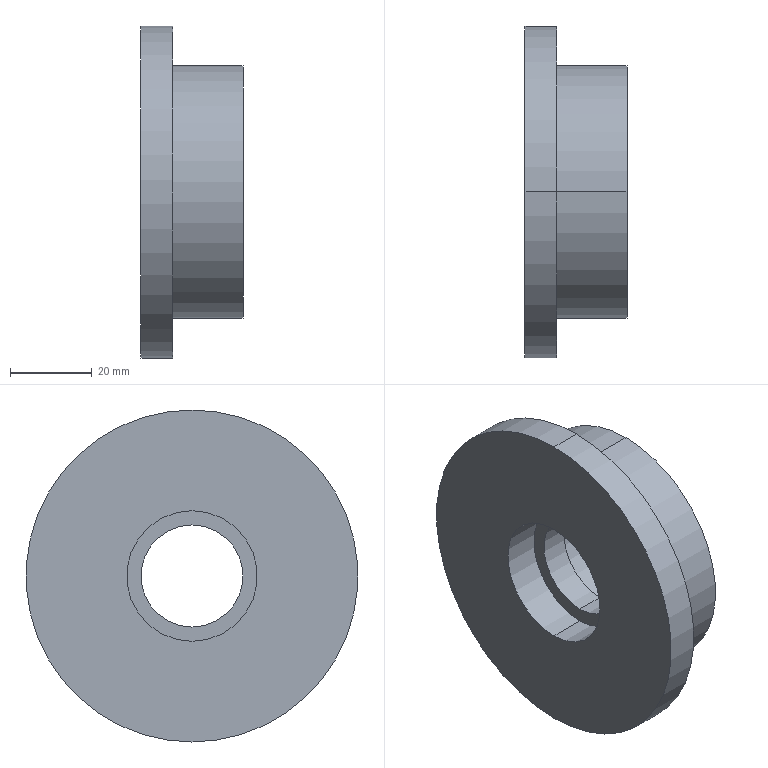Part | STEP file | PN_0073 (sprocket z=16,p=15.875) | 1 solid | 15 faces | box 25 x 81.37 x 81.37 mm | volume 74577 mm3 | cylinder 10 | plane 5 | commonest cylinder face diameters 32 x4 25 x2 62 x2 81.37 x2
STEP:
#1=CARTESIAN_POINT('',(0.,0.,0.));
#2=DIRECTION('',(0.,0.,1.));
#3=DIRECTION('',(1.,0.,0.));
#4=AXIS2_PLACEMENT_3D('',#1,#2,#3);
#5=CARTESIAN_POINT('',(9.,0.,16.));
#6=VERTEX_POINT('',#5);
#7=CARTESIAN_POINT('',(0.,0.,16.));
#8=VERTEX_POINT('',#7);
#9=CARTESIAN_POINT('',(9.,0.,16.));
#10=DIRECTION('',(-1.,0.,0.));
#11=VECTOR('',#10,1.);
#12=LINE('',#9,#11);
#13=CARTESIAN_POINT('',(9.,0.,0.));
#14=DIRECTION('',(-1.,0.,0.));
#15=DIRECTION('',(0.,0.,1.));
#16=AXIS2_PLACEMENT_3D('',#13,#14,#15);
#17=CYLINDRICAL_SURFACE('',#16,16.);
#18=CARTESIAN_POINT('',(6.283,0.));
#19=DIRECTION('',(0.,1.));
#20=VECTOR('',#19,1.);
#21=LINE('',#18,#20);
#22=(GEOMETRIC_REPRESENTATION_CONTEXT(2)PARAMETRIC_REPRESENTATION_CONTEXT()REPRESENTATION_CONTEXT('',''));
#23=DEFINITIONAL_REPRESENTATION('',(#21),#22);
#24=PCURVE('',#17,#23);
#25=CARTESIAN_POINT('',(9.,0.,0.));
#26=DIRECTION('',(-1.,0.,0.));
#27=DIRECTION('',(0.,0.,1.));
#28=AXIS2_PLACEMENT_3D('',#25,#26,#27);
#29=CYLINDRICAL_SURFACE('',#28,16.);
#30=CARTESIAN_POINT('',(0.,0.));
#31=DIRECTION('',(0.,1.));
#32=VECTOR('',#31,1.);
#33=LINE('',#30,#32);
#34=(GEOMETRIC_REPRESENTATION_CONTEXT(2)PARAMETRIC_REPRESENTATION_CONTEXT()REPRESENTATION_CONTEXT('',''));
#35=DEFINITIONAL_REPRESENTATION('',(#33),#34);
#36=PCURVE('',#29,#35);
#37=SURFACE_CURVE('',#12,(#24,#36),.PCURVE_S1.);
#38=EDGE_CURVE('',#6,#8,#37,.T.);
#39=ORIENTED_EDGE('',*,*,#38,.T.);
#40=CARTESIAN_POINT('',(0.,0.,-16.));
#41=VERTEX_POINT('',#40);
#42=CARTESIAN_POINT('',(0.,0.,0.));
#43=DIRECTION('',(-1.,0.,0.));
#44=DIRECTION('',(0.,0.,1.));
#45=AXIS2_PLACEMENT_3D('',#42,#43,#44);
#46=CIRCLE('',#45,16.);
#47=CARTESIAN_POINT('',(0.,9.));
#48=DIRECTION('',(1.,0.));
#49=VECTOR('',#48,1.);
#50=LINE('',#47,#49);
#51=(GEOMETRIC_REPRESENTATION_CONTEXT(2)PARAMETRIC_REPRESENTATION_CONTEXT()REPRESENTATION_CONTEXT('',''));
#52=DEFINITIONAL_REPRESENTATION('',(#50),#51);
#53=PCURVE('',#17,#52);
#54=CARTESIAN_POINT('',(0.,0.,0.));
#55=DIRECTION('',(1.,0.,0.));
#56=DIRECTION('',(0.,0.,-1.));
#57=AXIS2_PLACEMENT_3D('',#54,#55,#56);
#58=PLANE('',#57);
#59=CARTESIAN_POINT('',(-16.,0.));
#60=CARTESIAN_POINT('',(-16.,27.713));
#61=CARTESIAN_POINT('',(8.,13.856));
#62=CARTESIAN_POINT('',(32.,0.));
#63=CARTESIAN_POINT('',(8.,-13.856));
#64=CARTESIAN_POINT('',(-16.,-27.713));
#65=CARTESIAN_POINT('',(-16.,0.));
#66=(BOUNDED_CURVE()B_SPLINE_CURVE(2,(#59,#60,#61,#62,#63,#64,#65),.UNSPECIFIED.,.T.,.F.)B_SPLINE_CURVE_WITH_KNOTS((1,2,2,2,2,1),(-2.094,0.,2.094,4.189,6.283,8.378),.UNSPECIFIED.)CURVE()GEOMETRIC_REPRESENTATION_ITEM()RATIONAL_B_SPLINE_CURVE((1.,0.5,1.,0.5,1.,0.5,1.))REPRESENTATION_ITEM(''));
#67=(GEOMETRIC_REPRESENTATION_CONTEXT(2)PARAMETRIC_REPRESENTATION_CONTEXT()REPRESENTATION_CONTEXT('',''));
#68=DEFINITIONAL_REPRESENTATION('',(#66),#67);
#69=PCURVE('',#58,#68);
#70=SURFACE_CURVE('',#46,(#53,#69),.PCURVE_S1.);
#71=EDGE_CURVE('',#41,#8,#70,.T.);
#72=ORIENTED_EDGE('',*,*,#71,.F.);
#73=CARTESIAN_POINT('',(9.,0.,-16.));
#74=VERTEX_POINT('',#73);
#75=CARTESIAN_POINT('',(9.,0.,-16.));
#76=DIRECTION('',(-1.,0.,0.));
#77=VECTOR('',#76,1.);
#78=LINE('',#75,#77);
#79=CARTESIAN_POINT('',(3.142,0.));
#80=DIRECTION('',(0.,1.));
#81=VECTOR('',#80,1.);
#82=LINE('',#79,#81);
#83=(GEOMETRIC_REPRESENTATION_CONTEXT(2)PARAMETRIC_REPRESENTATION_CONTEXT()REPRESENTATION_CONTEXT('',''));
#84=DEFINITIONAL_REPRESENTATION('',(#82),#83);
#85=PCURVE('',#17,#84);
#86=CARTESIAN_POINT('',(3.142,0.));
#87=DIRECTION('',(0.,1.));
#88=VECTOR('',#87,1.);
#89=LINE('',#86,#88);
#90=(GEOMETRIC_REPRESENTATION_CONTEXT(2)PARAMETRIC_REPRESENTATION_CONTEXT()REPRESENTATION_CONTEXT('',''));
#91=DEFINITIONAL_REPRESENTATION('',(#89),#90);
#92=PCURVE('',#29,#91);
#93=SURFACE_CURVE('',#78,(#85,#92),.PCURVE_S1.);
#94=EDGE_CURVE('',#74,#41,#93,.T.);
#95=ORIENTED_EDGE('',*,*,#94,.F.);
#96=CARTESIAN_POINT('',(9.,0.,0.));
#97=DIRECTION('',(-1.,0.,0.));
#98=DIRECTION('',(0.,0.,1.));
#99=AXIS2_PLACEMENT_3D('',#96,#97,#98);
#100=CIRCLE('',#99,16.);
#101=CARTESIAN_POINT('',(0.,0.));
#102=DIRECTION('',(1.,0.));
#103=VECTOR('',#102,1.);
#104=LINE('',#101,#103);
#105=(GEOMETRIC_REPRESENTATION_CONTEXT(2)PARAMETRIC_REPRESENTATION_CONTEXT()REPRESENTATION_CONTEXT('',''));
#106=DEFINITIONAL_REPRESENTATION('',(#104),#105);
#107=PCURVE('',#17,#106);
#108=CARTESIAN_POINT('',(9.,0.,0.));
#109=DIRECTION('',(-1.,0.,0.));
#110=DIRECTION('',(0.,0.,1.));
#111=AXIS2_PLACEMENT_3D('',#108,#109,#110);
#112=PLANE('',#111);
#113=CARTESIAN_POINT('',(0.,0.));
#114=DIRECTION('',(1.,0.));
#115=AXIS2_PLACEMENT_2D('',#113,#114);
#116=CIRCLE('',#115,16.);
#117=(GEOMETRIC_REPRESENTATION_CONTEXT(2)PARAMETRIC_REPRESENTATION_CONTEXT()REPRESENTATION_CONTEXT('',''));
#118=DEFINITIONAL_REPRESENTATION('',(#116),#117);
#119=PCURVE('',#112,#118);
#120=SURFACE_CURVE('',#100,(#107,#119),.PCURVE_S1.);
#121=EDGE_CURVE('',#74,#6,#120,.T.);
#122=ORIENTED_EDGE('',*,*,#121,.T.);
#123=EDGE_LOOP('',(#39,#72,#95,#122));
#124=FACE_BOUND('',#123,.F.);
#125=ADVANCED_FACE('',(#124),#17,.F.);
#126=CARTESIAN_POINT('',(16.,0.,-16.));
#127=VERTEX_POINT('',#126);
#128=CARTESIAN_POINT('',(25.,0.,-16.));
#129=VERTEX_POINT('',#128);
#130=CARTESIAN_POINT('',(16.,0.,-16.));
#131=DIRECTION('',(1.,0.,0.));
#132=VECTOR('',#131,1.);
#133=LINE('',#130,#132);
#134=CARTESIAN_POINT('',(16.,0.,0.));
#135=DIRECTION('',(1.,0.,0.));
#136=DIRECTION('',(0.,0.,-1.));
#137=AXIS2_PLACEMENT_3D('',#134,#135,#136);
#138=CYLINDRICAL_SURFACE('',#137,16.);
#139=CARTESIAN_POINT('',(6.283,0.));
#140=DIRECTION('',(0.,1.));
#141=VECTOR('',#140,1.);
#142=LINE('',#139,#141);
#143=(GEOMETRIC_REPRESENTATION_CONTEXT(2)PARAMETRIC_REPRESENTATION_CONTEXT()REPRESENTATION_CONTEXT('',''));
#144=DEFINITIONAL_REPRESENTATION('',(#142),#143);
#145=PCURVE('',#138,#144);
#146=CARTESIAN_POINT('',(16.,0.,0.));
#147=DIRECTION('',(1.,0.,0.));
#148=DIRECTION('',(0.,0.,-1.));
#149=AXIS2_PLACEMENT_3D('',#146,#147,#148);
#150=CYLINDRICAL_SURFACE('',#149,16.);
#151=CARTESIAN_POINT('',(0.,0.));
#152=DIRECTION('',(0.,1.));
#153=VECTOR('',#152,1.);
#154=LINE('',#151,#153);
#155=(GEOMETRIC_REPRESENTATION_CONTEXT(2)PARAMETRIC_REPRESENTATION_CONTEXT()REPRESENTATION_CONTEXT('',''));
#156=DEFINITIONAL_REPRESENTATION('',(#154),#155);
#157=PCURVE('',#150,#156);
#158=SURFACE_CURVE('',#133,(#145,#157),.PCURVE_S1.);
#159=EDGE_CURVE('',#127,#129,#158,.T.);
#160=ORIENTED_EDGE('',*,*,#159,.T.);
#161=CARTESIAN_POINT('',(25.,0.,16.));
#162=VERTEX_POINT('',#161);
#163=CARTESIAN_POINT('',(25.,0.,0.));
#164=DIRECTION('',(1.,0.,0.));
#165=DIRECTION('',(0.,0.,-1.));
#166=AXIS2_PLACEMENT_3D('',#163,#164,#165);
#167=CIRCLE('',#166,16.);
#168=CARTESIAN_POINT('',(0.,9.));
#169=DIRECTION('',(1.,0.));
#170=VECTOR('',#169,1.);
#171=LINE('',#168,#170);
#172=(GEOMETRIC_REPRESENTATION_CONTEXT(2)PARAMETRIC_REPRESENTATION_CONTEXT()REPRESENTATION_CONTEXT('',''));
#173=DEFINITIONAL_REPRESENTATION('',(#171),#172);
#174=PCURVE('',#138,#173);
#175=CARTESIAN_POINT('',(25.,0.,0.));
#176=DIRECTION('',(1.,0.,0.));
#177=DIRECTION('',(0.,0.,-1.));
#178=AXIS2_PLACEMENT_3D('',#175,#176,#177);
#179=PLANE('',#178);
#180=CARTESIAN_POINT('',(0.,0.));
#181=DIRECTION('',(1.,0.));
#182=AXIS2_PLACEMENT_2D('',#180,#181);
#183=CIRCLE('',#182,16.);
#184=(GEOMETRIC_REPRESENTATION_CONTEXT(2)PARAMETRIC_REPRESENTATION_CONTEXT()REPRESENTATION_CONTEXT('',''));
#185=DEFINITIONAL_REPRESENTATION('',(#183),#184);
#186=PCURVE('',#179,#185);
#187=SURFACE_CURVE('',#167,(#174,#186),.PCURVE_S1.);
#188=EDGE_CURVE('',#162,#129,#187,.T.);
#189=ORIENTED_EDGE('',*,*,#188,.F.);
#190=CARTESIAN_POINT('',(16.,0.,16.));
#191=VERTEX_POINT('',#190);
#192=CARTESIAN_POINT('',(16.,0.,16.));
#193=DIRECTION('',(1.,0.,0.));
#194=VECTOR('',#193,1.);
#195=LINE('',#192,#194);
#196=CARTESIAN_POINT('',(3.142,0.));
#197=DIRECTION('',(0.,1.));
#198=VECTOR('',#197,1.);
#199=LINE('',#196,#198);
#200=(GEOMETRIC_REPRESENTATION_CONTEXT(2)PARAMETRIC_REPRESENTATION_CONTEXT()REPRESENTATION_CONTEXT('',''));
#201=DEFINITIONAL_REPRESENTATION('',(#199),#200);
#202=PCURVE('',#138,#201);
#203=CARTESIAN_POINT('',(3.142,0.));
#204=DIRECTION('',(0.,1.));
#205=VECTOR('',#204,1.);
#206=LINE('',#203,#205);
#207=(GEOMETRIC_REPRESENTATION_CONTEXT(2)PARAMETRIC_REPRESENTATION_CONTEXT()REPRESENTATION_CONTEXT('',''));
#208=DEFINITIONAL_REPRESENTATION('',(#206),#207);
#209=PCURVE('',#150,#208);
#210=SURFACE_CURVE('',#195,(#202,#209),.PCURVE_S1.);
#211=EDGE_CURVE('',#191,#162,#210,.T.);
#212=ORIENTED_EDGE('',*,*,#211,.F.);
#213=CARTESIAN_POINT('',(16.,0.,0.));
#214=DIRECTION('',(1.,0.,0.));
#215=DIRECTION('',(0.,0.,-1.));
#216=AXIS2_PLACEMENT_3D('',#213,#214,#215);
#217=CIRCLE('',#216,16.);
#218=CARTESIAN_POINT('',(0.,0.));
#219=DIRECTION('',(1.,0.));
#220=VECTOR('',#219,1.);
#221=LINE('',#218,#220);
#222=(GEOMETRIC_REPRESENTATION_CONTEXT(2)PARAMETRIC_REPRESENTATION_CONTEXT()REPRESENTATION_CONTEXT('',''));
#223=DEFINITIONAL_REPRESENTATION('',(#221),#222);
#224=PCURVE('',#138,#223);
#225=CARTESIAN_POINT('',(16.,0.,0.));
#226=DIRECTION('',(1.,0.,0.));
#227=DIRECTION('',(0.,0.,-1.));
#228=AXIS2_PLACEMENT_3D('',#225,#226,#227);
#229=PLANE('',#228);
#230=CARTESIAN_POINT('',(0.,0.));
#231=DIRECTION('',(1.,0.));
#232=AXIS2_PLACEMENT_2D('',#230,#231);
#233=CIRCLE('',#232,16.);
#234=(GEOMETRIC_REPRESENTATION_CONTEXT(2)PARAMETRIC_REPRESENTATION_CONTEXT()REPRESENTATION_CONTEXT('',''));
#235=DEFINITIONAL_REPRESENTATION('',(#233),#234);
#236=PCURVE('',#229,#235);
#237=SURFACE_CURVE('',#217,(#224,#236),.PCURVE_S1.);
#238=EDGE_CURVE('',#191,#127,#237,.T.);
#239=ORIENTED_EDGE('',*,*,#238,.T.);
#240=EDGE_LOOP('',(#160,#189,#212,#239));
#241=FACE_BOUND('',#240,.F.);
#242=ADVANCED_FACE('',(#241),#138,.F.);
#243=CARTESIAN_POINT('',(25.,0.,-31.));
#244=VERTEX_POINT('',#243);
#245=CARTESIAN_POINT('',(25.,0.,31.));
#246=VERTEX_POINT('',#245);
#247=CARTESIAN_POINT('',(25.,0.,0.));
#248=DIRECTION('',(1.,0.,0.));
#249=DIRECTION('',(0.,0.,-1.));
#250=AXIS2_PLACEMENT_3D('',#247,#248,#249);
#251=CIRCLE('',#250,31.);
#252=CARTESIAN_POINT('',(25.,0.,0.));
#253=DIRECTION('',(-1.,0.,0.));
#254=DIRECTION('',(0.,0.,1.));
#255=AXIS2_PLACEMENT_3D('',#252,#253,#254);
#256=CYLINDRICAL_SURFACE('',#255,31.);
#257=CARTESIAN_POINT('',(3.142,0.));
#258=DIRECTION('',(-1.,0.));
#259=VECTOR('',#258,1.);
#260=LINE('',#257,#259);
#261=(GEOMETRIC_REPRESENTATION_CONTEXT(2)PARAMETRIC_REPRESENTATION_CONTEXT()REPRESENTATION_CONTEXT('',''));
#262=DEFINITIONAL_REPRESENTATION('',(#260),#261);
#263=PCURVE('',#256,#262);
#264=CARTESIAN_POINT('',(0.,0.));
#265=DIRECTION('',(1.,0.));
#266=AXIS2_PLACEMENT_2D('',#264,#265);
#267=CIRCLE('',#266,31.);
#268=(GEOMETRIC_REPRESENTATION_CONTEXT(2)PARAMETRIC_REPRESENTATION_CONTEXT()REPRESENTATION_CONTEXT('',''));
#269=DEFINITIONAL_REPRESENTATION('',(#267),#268);
#270=PCURVE('',#179,#269);
#271=SURFACE_CURVE('',#251,(#263,#270),.PCURVE_S1.);
#272=EDGE_CURVE('',#244,#246,#271,.T.);
#273=ORIENTED_EDGE('',*,*,#272,.F.);
#274=CARTESIAN_POINT('',(7.8,0.,-31.));
#275=VERTEX_POINT('',#274);
#276=CARTESIAN_POINT('',(25.,0.,-31.));
#277=DIRECTION('',(-1.,0.,0.));
#278=VECTOR('',#277,1.);
#279=LINE('',#276,#278);
#280=CARTESIAN_POINT('',(3.142,0.));
#281=DIRECTION('',(0.,1.));
#282=VECTOR('',#281,1.);
#283=LINE('',#280,#282);
#284=(GEOMETRIC_REPRESENTATION_CONTEXT(2)PARAMETRIC_REPRESENTATION_CONTEXT()REPRESENTATION_CONTEXT('',''));
#285=DEFINITIONAL_REPRESENTATION('',(#283),#284);
#286=PCURVE('',#256,#285);
#287=CARTESIAN_POINT('',(25.,0.,0.));
#288=DIRECTION('',(-1.,0.,0.));
#289=DIRECTION('',(0.,0.,1.));
#290=AXIS2_PLACEMENT_3D('',#287,#288,#289);
#291=CYLINDRICAL_SURFACE('',#290,31.);
#292=CARTESIAN_POINT('',(3.142,0.));
#293=DIRECTION('',(0.,1.));
#294=VECTOR('',#293,1.);
#295=LINE('',#292,#294);
#296=(GEOMETRIC_REPRESENTATION_CONTEXT(2)PARAMETRIC_REPRESENTATION_CONTEXT()REPRESENTATION_CONTEXT('',''));
#297=DEFINITIONAL_REPRESENTATION('',(#295),#296);
#298=PCURVE('',#291,#297);
#299=SURFACE_CURVE('',#279,(#286,#298),.PCURVE_S1.);
#300=EDGE_CURVE('',#244,#275,#299,.T.);
#301=ORIENTED_EDGE('',*,*,#300,.T.);
#302=CARTESIAN_POINT('',(7.8,0.,31.));
#303=VERTEX_POINT('',#302);
#304=CARTESIAN_POINT('',(7.8,0.,0.));
#305=DIRECTION('',(1.,0.,0.));
#306=DIRECTION('',(0.,0.,-1.));
#307=AXIS2_PLACEMENT_3D('',#304,#305,#306);
#308=CIRCLE('',#307,31.);
#309=CARTESIAN_POINT('',(3.142,17.2));
#310=DIRECTION('',(-1.,0.));
#311=VECTOR('',#310,1.);
#312=LINE('',#309,#311);
#313=(GEOMETRIC_REPRESENTATION_CONTEXT(2)PARAMETRIC_REPRESENTATION_CONTEXT()REPRESENTATION_CONTEXT('',''));
#314=DEFINITIONAL_REPRESENTATION('',(#312),#313);
#315=PCURVE('',#256,#314);
#316=CARTESIAN_POINT('',(7.8,0.,0.));
#317=DIRECTION('',(1.,0.,0.));
#318=DIRECTION('',(0.,0.,-1.));
#319=AXIS2_PLACEMENT_3D('',#316,#317,#318);
#320=PLANE('',#319);
#321=CARTESIAN_POINT('',(0.,0.));
#322=DIRECTION('',(1.,0.));
#323=AXIS2_PLACEMENT_2D('',#321,#322);
#324=CIRCLE('',#323,31.);
#325=(GEOMETRIC_REPRESENTATION_CONTEXT(2)PARAMETRIC_REPRESENTATION_CONTEXT()REPRESENTATION_CONTEXT('',''));
#326=DEFINITIONAL_REPRESENTATION('',(#324),#325);
#327=PCURVE('',#320,#326);
#328=SURFACE_CURVE('',#308,(#315,#327),.PCURVE_S1.);
#329=EDGE_CURVE('',#275,#303,#328,.T.);
#330=ORIENTED_EDGE('',*,*,#329,.T.);
#331=CARTESIAN_POINT('',(25.,0.,31.));
#332=DIRECTION('',(-1.,0.,0.));
#333=VECTOR('',#332,1.);
#334=LINE('',#331,#333);
#335=CARTESIAN_POINT('',(0.,0.));
#336=DIRECTION('',(0.,1.));
#337=VECTOR('',#336,1.);
#338=LINE('',#335,#337);
#339=(GEOMETRIC_REPRESENTATION_CONTEXT(2)PARAMETRIC_REPRESENTATION_CONTEXT()REPRESENTATION_CONTEXT('',''));
#340=DEFINITIONAL_REPRESENTATION('',(#338),#339);
#341=PCURVE('',#256,#340);
#342=CARTESIAN_POINT('',(6.283,0.));
#343=DIRECTION('',(0.,1.));
#344=VECTOR('',#343,1.);
#345=LINE('',#342,#344);
#346=(GEOMETRIC_REPRESENTATION_CONTEXT(2)PARAMETRIC_REPRESENTATION_CONTEXT()REPRESENTATION_CONTEXT('',''));
#347=DEFINITIONAL_REPRESENTATION('',(#345),#346);
#348=PCURVE('',#291,#347);
#349=SURFACE_CURVE('',#334,(#341,#348),.PCURVE_S1.);
#350=EDGE_CURVE('',#246,#303,#349,.T.);
#351=ORIENTED_EDGE('',*,*,#350,.F.);
#352=EDGE_LOOP('',(#273,#301,#330,#351));
#353=FACE_BOUND('',#352,.T.);
#354=ADVANCED_FACE('',(#353),#256,.T.);
#355=CARTESIAN_POINT('',(7.8,0.,-40.685));
#356=VERTEX_POINT('',#355);
#357=CARTESIAN_POINT('',(7.8,0.,40.685));
#358=VERTEX_POINT('',#357);
#359=CARTESIAN_POINT('',(7.8,0.,0.));
#360=DIRECTION('',(1.,0.,0.));
#361=DIRECTION('',(0.,0.,-1.));
#362=AXIS2_PLACEMENT_3D('',#359,#360,#361);
#363=CIRCLE('',#362,40.685);
#364=CARTESIAN_POINT('',(7.8,0.,0.));
#365=DIRECTION('',(-1.,0.,0.));
#366=DIRECTION('',(0.,0.,1.));
#367=AXIS2_PLACEMENT_3D('',#364,#365,#366);
#368=CYLINDRICAL_SURFACE('',#367,40.685);
#369=CARTESIAN_POINT('',(3.142,0.));
#370=DIRECTION('',(-1.,0.));
#371=VECTOR('',#370,1.);
#372=LINE('',#369,#371);
#373=(GEOMETRIC_REPRESENTATION_CONTEXT(2)PARAMETRIC_REPRESENTATION_CONTEXT()REPRESENTATION_CONTEXT('',''));
#374=DEFINITIONAL_REPRESENTATION('',(#372),#373);
#375=PCURVE('',#368,#374);
#376=CARTESIAN_POINT('',(0.,0.));
#377=DIRECTION('',(1.,0.));
#378=AXIS2_PLACEMENT_2D('',#376,#377);
#379=CIRCLE('',#378,40.685);
#380=(GEOMETRIC_REPRESENTATION_CONTEXT(2)PARAMETRIC_REPRESENTATION_CONTEXT()REPRESENTATION_CONTEXT('',''));
#381=DEFINITIONAL_REPRESENTATION('',(#379),#380);
#382=PCURVE('',#320,#381);
#383=SURFACE_CURVE('',#363,(#375,#382),.PCURVE_S1.);
#384=EDGE_CURVE('',#356,#358,#383,.T.);
#385=ORIENTED_EDGE('',*,*,#384,.F.);
#386=CARTESIAN_POINT('',(0.,0.,-40.685));
#387=VERTEX_POINT('',#386);
#388=CARTESIAN_POINT('',(7.8,0.,-40.685));
#389=DIRECTION('',(-1.,0.,0.));
#390=VECTOR('',#389,1.);
#391=LINE('',#388,#390);
#392=CARTESIAN_POINT('',(3.142,0.));
#393=DIRECTION('',(0.,1.));
#394=VECTOR('',#393,1.);
#395=LINE('',#392,#394);
#396=(GEOMETRIC_REPRESENTATION_CONTEXT(2)PARAMETRIC_REPRESENTATION_CONTEXT()REPRESENTATION_CONTEXT('',''));
#397=DEFINITIONAL_REPRESENTATION('',(#395),#396);
#398=PCURVE('',#368,#397);
#399=CARTESIAN_POINT('',(7.8,0.,0.));
#400=DIRECTION('',(-1.,0.,0.));
#401=DIRECTION('',(0.,0.,1.));
#402=AXIS2_PLACEMENT_3D('',#399,#400,#401);
#403=CYLINDRICAL_SURFACE('',#402,40.685);
#404=CARTESIAN_POINT('',(3.142,0.));
#405=DIRECTION('',(0.,1.));
#406=VECTOR('',#405,1.);
#407=LINE('',#404,#406);
#408=(GEOMETRIC_REPRESENTATION_CONTEXT(2)PARAMETRIC_REPRESENTATION_CONTEXT()REPRESENTATION_CONTEXT('',''));
#409=DEFINITIONAL_REPRESENTATION('',(#407),#408);
#410=PCURVE('',#403,#409);
#411=SURFACE_CURVE('',#391,(#398,#410),.PCURVE_S1.);
#412=EDGE_CURVE('',#356,#387,#411,.T.);
#413=ORIENTED_EDGE('',*,*,#412,.T.);
#414=CARTESIAN_POINT('',(0.,0.,40.685));
#415=VERTEX_POINT('',#414);
#416=CARTESIAN_POINT('',(0.,0.,0.));
#417=DIRECTION('',(1.,0.,0.));
#418=DIRECTION('',(0.,0.,-1.));
#419=AXIS2_PLACEMENT_3D('',#416,#417,#418);
#420=CIRCLE('',#419,40.685);
#421=CARTESIAN_POINT('',(3.142,7.8));
#422=DIRECTION('',(-1.,0.));
#423=VECTOR('',#422,1.);
#424=LINE('',#421,#423);
#425=(GEOMETRIC_REPRESENTATION_CONTEXT(2)PARAMETRIC_REPRESENTATION_CONTEXT()REPRESENTATION_CONTEXT('',''));
#426=DEFINITIONAL_REPRESENTATION('',(#424),#425);
#427=PCURVE('',#368,#426);
#428=CARTESIAN_POINT('',(0.,0.));
#429=DIRECTION('',(1.,0.));
#430=AXIS2_PLACEMENT_2D('',#428,#429);
#431=CIRCLE('',#430,40.685);
#432=(GEOMETRIC_REPRESENTATION_CONTEXT(2)PARAMETRIC_REPRESENTATION_CONTEXT()REPRESENTATION_CONTEXT('',''));
#433=DEFINITIONAL_REPRESENTATION('',(#431),#432);
#434=PCURVE('',#58,#433);
#435=SURFACE_CURVE('',#420,(#427,#434),.PCURVE_S1.);
#436=EDGE_CURVE('',#387,#415,#435,.T.);
#437=ORIENTED_EDGE('',*,*,#436,.T.);
#438=CARTESIAN_POINT('',(7.8,0.,40.685));
#439=DIRECTION('',(-1.,0.,0.));
#440=VECTOR('',#439,1.);
#441=LINE('',#438,#440);
#442=CARTESIAN_POINT('',(0.,0.));
#443=DIRECTION('',(0.,1.));
#444=VECTOR('',#443,1.);
#445=LINE('',#442,#444);
#446=(GEOMETRIC_REPRESENTATION_CONTEXT(2)PARAMETRIC_REPRESENTATION_CONTEXT()REPRESENTATION_CONTEXT('',''));
#447=DEFINITIONAL_REPRESENTATION('',(#445),#446);
#448=PCURVE('',#368,#447);
#449=CARTESIAN_POINT('',(6.283,0.));
#450=DIRECTION('',(0.,1.));
#451=VECTOR('',#450,1.);
#452=LINE('',#449,#451);
#453=(GEOMETRIC_REPRESENTATION_CONTEXT(2)PARAMETRIC_REPRESENTATION_CONTEXT()REPRESENTATION_CONTEXT('',''));
#454=DEFINITIONAL_REPRESENTATION('',(#452),#453);
#455=PCURVE('',#403,#454);
#456=SURFACE_CURVE('',#441,(#448,#455),.PCURVE_S1.);
#457=EDGE_CURVE('',#358,#415,#456,.T.);
#458=ORIENTED_EDGE('',*,*,#457,.F.);
#459=EDGE_LOOP('',(#385,#413,#437,#458));
#460=FACE_BOUND('',#459,.T.);
#461=ADVANCED_FACE('',(#460),#368,.T.);
#462=CARTESIAN_POINT('',(9.,0.,-12.5));
#463=VERTEX_POINT('',#462);
#464=CARTESIAN_POINT('',(16.,0.,-12.5));
#465=VERTEX_POINT('',#464);
#466=CARTESIAN_POINT('',(0.,0.,-12.5));
#467=DIRECTION('',(1.,0.,0.));
#468=VECTOR('',#467,1.);
#469=LINE('',#466,#468);
#470=CARTESIAN_POINT('',(0.,0.,0.));
#471=DIRECTION('',(1.,0.,0.));
#472=DIRECTION('',(0.,0.,-1.));
#473=AXIS2_PLACEMENT_3D('',#470,#471,#472);
#474=CYLINDRICAL_SURFACE('',#473,12.5);
#475=CARTESIAN_POINT('',(6.283,0.));
#476=DIRECTION('',(0.,1.));
#477=VECTOR('',#476,1.);
#478=LINE('',#475,#477);
#479=(GEOMETRIC_REPRESENTATION_CONTEXT(2)PARAMETRIC_REPRESENTATION_CONTEXT()REPRESENTATION_CONTEXT('',''));
#480=DEFINITIONAL_REPRESENTATION('',(#478),#479);
#481=PCURVE('',#474,#480);
#482=CARTESIAN_POINT('',(0.,0.,0.));
#483=DIRECTION('',(1.,0.,0.));
#484=DIRECTION('',(0.,0.,-1.));
#485=AXIS2_PLACEMENT_3D('',#482,#483,#484);
#486=CYLINDRICAL_SURFACE('',#485,12.5);
#487=CARTESIAN_POINT('',(0.,0.));
#488=DIRECTION('',(0.,1.));
#489=VECTOR('',#488,1.);
#490=LINE('',#487,#489);
#491=(GEOMETRIC_REPRESENTATION_CONTEXT(2)PARAMETRIC_REPRESENTATION_CONTEXT()REPRESENTATION_CONTEXT('',''));
#492=DEFINITIONAL_REPRESENTATION('',(#490),#491);
#493=PCURVE('',#486,#492);
#494=SURFACE_CURVE('',#469,(#481,#493),.PCURVE_S1.);
#495=EDGE_CURVE('',#463,#465,#494,.T.);
#496=ORIENTED_EDGE('',*,*,#495,.T.);
#497=CARTESIAN_POINT('',(16.,0.,12.5));
#498=VERTEX_POINT('',#497);
#499=CARTESIAN_POINT('',(16.,0.,0.));
#500=DIRECTION('',(-1.,0.,0.));
#501=DIRECTION('',(0.,0.,-1.));
#502=AXIS2_PLACEMENT_3D('',#499,#500,#501);
#503=CIRCLE('',#502,12.5);
#504=CARTESIAN_POINT('',(6.283,16.));
#505=DIRECTION('',(-1.,0.));
#506=VECTOR('',#505,1.);
#507=LINE('',#504,#506);
#508=(GEOMETRIC_REPRESENTATION_CONTEXT(2)PARAMETRIC_REPRESENTATION_CONTEXT()REPRESENTATION_CONTEXT('',''));
#509=DEFINITIONAL_REPRESENTATION('',(#507),#508);
#510=PCURVE('',#474,#509);
#511=CARTESIAN_POINT('',(12.5,0.));
#512=CARTESIAN_POINT('',(12.5,-21.651));
#513=CARTESIAN_POINT('',(-6.25,-10.825));
#514=CARTESIAN_POINT('',(-25.,0.));
#515=CARTESIAN_POINT('',(-6.25,10.825));
#516=CARTESIAN_POINT('',(12.5,21.651));
#517=CARTESIAN_POINT('',(12.5,0.));
#518=(BOUNDED_CURVE()B_SPLINE_CURVE(2,(#511,#512,#513,#514,#515,#516,#517),.UNSPECIFIED.,.T.,.F.)B_SPLINE_CURVE_WITH_KNOTS((1,2,2,2,2,1),(-2.094,0.,2.094,4.189,6.283,8.378),.UNSPECIFIED.)CURVE()GEOMETRIC_REPRESENTATION_ITEM()RATIONAL_B_SPLINE_CURVE((1.,0.5,1.,0.5,1.,0.5,1.))REPRESENTATION_ITEM(''));
#519=(GEOMETRIC_REPRESENTATION_CONTEXT(2)PARAMETRIC_REPRESENTATION_CONTEXT()REPRESENTATION_CONTEXT('',''));
#520=DEFINITIONAL_REPRESENTATION('',(#518),#519);
#521=PCURVE('',#229,#520);
#522=SURFACE_CURVE('',#503,(#510,#521),.PCURVE_S1.);
#523=EDGE_CURVE('',#465,#498,#522,.T.);
#524=ORIENTED_EDGE('',*,*,#523,.T.);
#525=CARTESIAN_POINT('',(9.,0.,12.5));
#526=VERTEX_POINT('',#525);
#527=CARTESIAN_POINT('',(0.,0.,12.5));
#528=DIRECTION('',(1.,0.,0.));
#529=VECTOR('',#528,1.);
#530=LINE('',#527,#529);
#531=CARTESIAN_POINT('',(3.142,0.));
#532=DIRECTION('',(0.,1.));
#533=VECTOR('',#532,1.);
#534=LINE('',#531,#533);
#535=(GEOMETRIC_REPRESENTATION_CONTEXT(2)PARAMETRIC_REPRESENTATION_CONTEXT()REPRESENTATION_CONTEXT('',''));
#536=DEFINITIONAL_REPRESENTATION('',(#534),#535);
#537=PCURVE('',#474,#536);
#538=CARTESIAN_POINT('',(3.142,0.));
#539=DIRECTION('',(0.,1.));
#540=VECTOR('',#539,1.);
#541=LINE('',#538,#540);
#542=(GEOMETRIC_REPRESENTATION_CONTEXT(2)PARAMETRIC_REPRESENTATION_CONTEXT()REPRESENTATION_CONTEXT('',''));
#543=DEFINITIONAL_REPRESENTATION('',(#541),#542);
#544=PCURVE('',#486,#543);
#545=SURFACE_CURVE('',#530,(#537,#544),.PCURVE_S1.);
#546=EDGE_CURVE('',#526,#498,#545,.T.);
#547=ORIENTED_EDGE('',*,*,#546,.F.);
#548=CARTESIAN_POINT('',(9.,0.,0.));
#549=DIRECTION('',(1.,0.,0.));
#550=DIRECTION('',(0.,0.,1.));
#551=AXIS2_PLACEMENT_3D('',#548,#549,#550);
#552=CIRCLE('',#551,12.5);
#553=CARTESIAN_POINT('',(3.142,9.));
#554=DIRECTION('',(1.,0.));
#555=VECTOR('',#554,1.);
#556=LINE('',#553,#555);
#557=(GEOMETRIC_REPRESENTATION_CONTEXT(2)PARAMETRIC_REPRESENTATION_CONTEXT()REPRESENTATION_CONTEXT('',''));
#558=DEFINITIONAL_REPRESENTATION('',(#556),#557);
#559=PCURVE('',#474,#558);
#560=CARTESIAN_POINT('',(12.5,0.));
#561=CARTESIAN_POINT('',(12.5,-21.651));
#562=CARTESIAN_POINT('',(-6.25,-10.825));
#563=CARTESIAN_POINT('',(-25.,0.));
#564=CARTESIAN_POINT('',(-6.25,10.825));
#565=CARTESIAN_POINT('',(12.5,21.651));
#566=CARTESIAN_POINT('',(12.5,0.));
#567=(BOUNDED_CURVE()B_SPLINE_CURVE(2,(#560,#561,#562,#563,#564,#565,#566),.UNSPECIFIED.,.T.,.F.)B_SPLINE_CURVE_WITH_KNOTS((1,2,2,2,2,1),(-2.094,0.,2.094,4.189,6.283,8.378),.UNSPECIFIED.)CURVE()GEOMETRIC_REPRESENTATION_ITEM()RATIONAL_B_SPLINE_CURVE((1.,0.5,1.,0.5,1.,0.5,1.))REPRESENTATION_ITEM(''));
#568=(GEOMETRIC_REPRESENTATION_CONTEXT(2)PARAMETRIC_REPRESENTATION_CONTEXT()REPRESENTATION_CONTEXT('',''));
#569=DEFINITIONAL_REPRESENTATION('',(#567),#568);
#570=PCURVE('',#112,#569);
#571=SURFACE_CURVE('',#552,(#559,#570),.PCURVE_S1.);
#572=EDGE_CURVE('',#526,#463,#571,.T.);
#573=ORIENTED_EDGE('',*,*,#572,.T.);
#574=EDGE_LOOP('',(#496,#524,#547,#573));
#575=FACE_BOUND('',#574,.F.);
#576=ADVANCED_FACE('',(#575),#474,.F.);
#577=CARTESIAN_POINT('',(16.,0.,0.));
#578=DIRECTION('',(-1.,0.,0.));
#579=DIRECTION('',(0.,0.,-1.));
#580=AXIS2_PLACEMENT_3D('',#577,#578,#579);
#581=CIRCLE('',#580,12.5);
#582=CARTESIAN_POINT('',(6.283,16.));
#583=DIRECTION('',(-1.,0.));
#584=VECTOR('',#583,1.);
#585=LINE('',#582,#584);
#586=(GEOMETRIC_REPRESENTATION_CONTEXT(2)PARAMETRIC_REPRESENTATION_CONTEXT()REPRESENTATION_CONTEXT('',''));
#587=DEFINITIONAL_REPRESENTATION('',(#585),#586);
#588=PCURVE('',#486,#587);
#589=CARTESIAN_POINT('',(12.5,0.));
#590=CARTESIAN_POINT('',(12.5,-21.651));
#591=CARTESIAN_POINT('',(-6.25,-10.825));
#592=CARTESIAN_POINT('',(-25.,0.));
#593=CARTESIAN_POINT('',(-6.25,10.825));
#594=CARTESIAN_POINT('',(12.5,21.651));
#595=CARTESIAN_POINT('',(12.5,0.));
#596=(BOUNDED_CURVE()B_SPLINE_CURVE(2,(#589,#590,#591,#592,#593,#594,#595),.UNSPECIFIED.,.T.,.F.)B_SPLINE_CURVE_WITH_KNOTS((1,2,2,2,2,1),(-2.094,0.,2.094,4.189,6.283,8.378),.UNSPECIFIED.)CURVE()GEOMETRIC_REPRESENTATION_ITEM()RATIONAL_B_SPLINE_CURVE((1.,0.5,1.,0.5,1.,0.5,1.))REPRESENTATION_ITEM(''));
#597=(GEOMETRIC_REPRESENTATION_CONTEXT(2)PARAMETRIC_REPRESENTATION_CONTEXT()REPRESENTATION_CONTEXT('',''));
#598=DEFINITIONAL_REPRESENTATION('',(#596),#597);
#599=PCURVE('',#229,#598);
#600=SURFACE_CURVE('',#581,(#588,#599),.PCURVE_S1.);
#601=EDGE_CURVE('',#498,#465,#600,.T.);
#602=ORIENTED_EDGE('',*,*,#601,.T.);
#603=ORIENTED_EDGE('',*,*,#495,.F.);
#604=CARTESIAN_POINT('',(9.,0.,0.));
#605=DIRECTION('',(1.,0.,0.));
#606=DIRECTION('',(0.,0.,1.));
#607=AXIS2_PLACEMENT_3D('',#604,#605,#606);
#608=CIRCLE('',#607,12.5);
#609=CARTESIAN_POINT('',(-3.142,9.));
#610=DIRECTION('',(1.,0.));
#611=VECTOR('',#610,1.);
#612=LINE('',#609,#611);
#613=(GEOMETRIC_REPRESENTATION_CONTEXT(2)PARAMETRIC_REPRESENTATION_CONTEXT()REPRESENTATION_CONTEXT('',''));
#614=DEFINITIONAL_REPRESENTATION('',(#612),#613);
#615=PCURVE('',#486,#614);
#616=CARTESIAN_POINT('',(12.5,0.));
#617=CARTESIAN_POINT('',(12.5,-21.651));
#618=CARTESIAN_POINT('',(-6.25,-10.825));
#619=CARTESIAN_POINT('',(-25.,0.));
#620=CARTESIAN_POINT('',(-6.25,10.825));
#621=CARTESIAN_POINT('',(12.5,21.651));
#622=CARTESIAN_POINT('',(12.5,0.));
#623=(BOUNDED_CURVE()B_SPLINE_CURVE(2,(#616,#617,#618,#619,#620,#621,#622),.UNSPECIFIED.,.T.,.F.)B_SPLINE_CURVE_WITH_KNOTS((1,2,2,2,2,1),(-2.094,0.,2.094,4.189,6.283,8.378),.UNSPECIFIED.)CURVE()GEOMETRIC_REPRESENTATION_ITEM()RATIONAL_B_SPLINE_CURVE((1.,0.5,1.,0.5,1.,0.5,1.))REPRESENTATION_ITEM(''));
#624=(GEOMETRIC_REPRESENTATION_CONTEXT(2)PARAMETRIC_REPRESENTATION_CONTEXT()REPRESENTATION_CONTEXT('',''));
#625=DEFINITIONAL_REPRESENTATION('',(#623),#624);
#626=PCURVE('',#112,#625);
#627=SURFACE_CURVE('',#608,(#615,#626),.PCURVE_S1.);
#628=EDGE_CURVE('',#463,#526,#627,.T.);
#629=ORIENTED_EDGE('',*,*,#628,.T.);
#630=ORIENTED_EDGE('',*,*,#546,.T.);
#631=EDGE_LOOP('',(#602,#603,#629,#630));
#632=FACE_BOUND('',#631,.F.);
#633=ADVANCED_FACE('',(#632),#486,.F.);
#634=CARTESIAN_POINT('',(7.8,0.,0.));
#635=DIRECTION('',(1.,0.,0.));
#636=DIRECTION('',(0.,0.,-1.));
#637=AXIS2_PLACEMENT_3D('',#634,#635,#636);
#638=CIRCLE('',#637,40.685);
#639=CARTESIAN_POINT('',(0.,0.));
#640=DIRECTION('',(1.,0.));
#641=AXIS2_PLACEMENT_2D('',#639,#640);
#642=CIRCLE('',#641,40.685);
#643=(GEOMETRIC_REPRESENTATION_CONTEXT(2)PARAMETRIC_REPRESENTATION_CONTEXT()REPRESENTATION_CONTEXT('',''));
#644=DEFINITIONAL_REPRESENTATION('',(#642),#643);
#645=PCURVE('',#320,#644);
#646=CARTESIAN_POINT('',(9.425,0.));
#647=DIRECTION('',(-1.,0.));
#648=VECTOR('',#647,1.);
#649=LINE('',#646,#648);
#650=(GEOMETRIC_REPRESENTATION_CONTEXT(2)PARAMETRIC_REPRESENTATION_CONTEXT()REPRESENTATION_CONTEXT('',''));
#651=DEFINITIONAL_REPRESENTATION('',(#649),#650);
#652=PCURVE('',#403,#651);
#653=SURFACE_CURVE('',#638,(#645,#652),.PCURVE_S1.);
#654=EDGE_CURVE('',#358,#356,#653,.T.);
#655=ORIENTED_EDGE('',*,*,#654,.T.);
#656=ORIENTED_EDGE('',*,*,#384,.T.);
#657=EDGE_LOOP('',(#655,#656));
#658=FACE_BOUND('',#657,.T.);
#659=CARTESIAN_POINT('',(7.8,0.,0.));
#660=DIRECTION('',(1.,0.,0.));
#661=DIRECTION('',(0.,0.,-1.));
#662=AXIS2_PLACEMENT_3D('',#659,#660,#661);
#663=CIRCLE('',#662,31.);
#664=CARTESIAN_POINT('',(0.,0.));
#665=DIRECTION('',(1.,0.));
#666=AXIS2_PLACEMENT_2D('',#664,#665);
#667=CIRCLE('',#666,31.);
#668=(GEOMETRIC_REPRESENTATION_CONTEXT(2)PARAMETRIC_REPRESENTATION_CONTEXT()REPRESENTATION_CONTEXT('',''));
#669=DEFINITIONAL_REPRESENTATION('',(#667),#668);
#670=PCURVE('',#320,#669);
#671=CARTESIAN_POINT('',(9.425,17.2));
#672=DIRECTION('',(-1.,0.));
#673=VECTOR('',#672,1.);
#674=LINE('',#671,#673);
#675=(GEOMETRIC_REPRESENTATION_CONTEXT(2)PARAMETRIC_REPRESENTATION_CONTEXT()REPRESENTATION_CONTEXT('',''));
#676=DEFINITIONAL_REPRESENTATION('',(#674),#675);
#677=PCURVE('',#291,#676);
#678=SURFACE_CURVE('',#663,(#670,#677),.PCURVE_S1.);
#679=EDGE_CURVE('',#303,#275,#678,.T.);
#680=ORIENTED_EDGE('',*,*,#679,.F.);
#681=ORIENTED_EDGE('',*,*,#329,.F.);
#682=EDGE_LOOP('',(#680,#681));
#683=FACE_BOUND('',#682,.T.);
#684=ADVANCED_FACE('',(#658,#683),#320,.T.);
#685=ORIENTED_EDGE('',*,*,#412,.F.);
#686=ORIENTED_EDGE('',*,*,#654,.F.);
#687=ORIENTED_EDGE('',*,*,#457,.T.);
#688=CARTESIAN_POINT('',(0.,0.,0.));
#689=DIRECTION('',(1.,0.,0.));
#690=DIRECTION('',(0.,0.,-1.));
#691=AXIS2_PLACEMENT_3D('',#688,#689,#690);
#692=CIRCLE('',#691,40.685);
#693=CARTESIAN_POINT('',(9.425,7.8));
#694=DIRECTION('',(-1.,0.));
#695=VECTOR('',#694,1.);
#696=LINE('',#693,#695);
#697=(GEOMETRIC_REPRESENTATION_CONTEXT(2)PARAMETRIC_REPRESENTATION_CONTEXT()REPRESENTATION_CONTEXT('',''));
#698=DEFINITIONAL_REPRESENTATION('',(#696),#697);
#699=PCURVE('',#403,#698);
#700=CARTESIAN_POINT('',(0.,0.));
#701=DIRECTION('',(1.,0.));
#702=AXIS2_PLACEMENT_2D('',#700,#701);
#703=CIRCLE('',#702,40.685);
#704=(GEOMETRIC_REPRESENTATION_CONTEXT(2)PARAMETRIC_REPRESENTATION_CONTEXT()REPRESENTATION_CONTEXT('',''));
#705=DEFINITIONAL_REPRESENTATION('',(#703),#704);
#706=PCURVE('',#58,#705);
#707=SURFACE_CURVE('',#692,(#699,#706),.PCURVE_S1.);
#708=EDGE_CURVE('',#415,#387,#707,.T.);
#709=ORIENTED_EDGE('',*,*,#708,.T.);
#710=EDGE_LOOP('',(#685,#686,#687,#709));
#711=FACE_BOUND('',#710,.T.);
#712=ADVANCED_FACE('',(#711),#403,.T.);
#713=CARTESIAN_POINT('',(0.,0.,0.));
#714=DIRECTION('',(-1.,0.,0.));
#715=DIRECTION('',(0.,0.,1.));
#716=AXIS2_PLACEMENT_3D('',#713,#714,#715);
#717=CIRCLE('',#716,16.);
#718=CARTESIAN_POINT('',(-16.,0.));
#719=CARTESIAN_POINT('',(-16.,27.713));
#720=CARTESIAN_POINT('',(8.,13.856));
#721=CARTESIAN_POINT('',(32.,0.));
#722=CARTESIAN_POINT('',(8.,-13.856));
#723=CARTESIAN_POINT('',(-16.,-27.713));
#724=CARTESIAN_POINT('',(-16.,0.));
#725=(BOUNDED_CURVE()B_SPLINE_CURVE(2,(#718,#719,#720,#721,#722,#723,#724),.UNSPECIFIED.,.T.,.F.)B_SPLINE_CURVE_WITH_KNOTS((1,2,2,2,2,1),(-2.094,0.,2.094,4.189,6.283,8.378),.UNSPECIFIED.)CURVE()GEOMETRIC_REPRESENTATION_ITEM()RATIONAL_B_SPLINE_CURVE((1.,0.5,1.,0.5,1.,0.5,1.))REPRESENTATION_ITEM(''));
#726=(GEOMETRIC_REPRESENTATION_CONTEXT(2)PARAMETRIC_REPRESENTATION_CONTEXT()REPRESENTATION_CONTEXT('',''));
#727=DEFINITIONAL_REPRESENTATION('',(#725),#726);
#728=PCURVE('',#58,#727);
#729=CARTESIAN_POINT('',(0.,9.));
#730=DIRECTION('',(1.,0.));
#731=VECTOR('',#730,1.);
#732=LINE('',#729,#731);
#733=(GEOMETRIC_REPRESENTATION_CONTEXT(2)PARAMETRIC_REPRESENTATION_CONTEXT()REPRESENTATION_CONTEXT('',''));
#734=DEFINITIONAL_REPRESENTATION('',(#732),#733);
#735=PCURVE('',#29,#734);
#736=SURFACE_CURVE('',#717,(#728,#735),.PCURVE_S1.);
#737=EDGE_CURVE('',#8,#41,#736,.T.);
#738=ORIENTED_EDGE('',*,*,#737,.F.);
#739=ORIENTED_EDGE('',*,*,#71,.F.);
#740=EDGE_LOOP('',(#738,#739));
#741=FACE_BOUND('',#740,.T.);
#742=ORIENTED_EDGE('',*,*,#708,.F.);
#743=ORIENTED_EDGE('',*,*,#436,.F.);
#744=EDGE_LOOP('',(#742,#743));
#745=FACE_BOUND('',#744,.T.);
#746=ADVANCED_FACE('',(#741,#745),#58,.F.);
#747=ORIENTED_EDGE('',*,*,#300,.F.);
#748=CARTESIAN_POINT('',(25.,0.,0.));
#749=DIRECTION('',(1.,0.,0.));
#750=DIRECTION('',(0.,0.,-1.));
#751=AXIS2_PLACEMENT_3D('',#748,#749,#750);
#752=CIRCLE('',#751,31.);
#753=CARTESIAN_POINT('',(9.425,0.));
#754=DIRECTION('',(-1.,0.));
#755=VECTOR('',#754,1.);
#756=LINE('',#753,#755);
#757=(GEOMETRIC_REPRESENTATION_CONTEXT(2)PARAMETRIC_REPRESENTATION_CONTEXT()REPRESENTATION_CONTEXT('',''));
#758=DEFINITIONAL_REPRESENTATION('',(#756),#757);
#759=PCURVE('',#291,#758);
#760=CARTESIAN_POINT('',(0.,0.));
#761=DIRECTION('',(1.,0.));
#762=AXIS2_PLACEMENT_2D('',#760,#761);
#763=CIRCLE('',#762,31.);
#764=(GEOMETRIC_REPRESENTATION_CONTEXT(2)PARAMETRIC_REPRESENTATION_CONTEXT()REPRESENTATION_CONTEXT('',''));
#765=DEFINITIONAL_REPRESENTATION('',(#763),#764);
#766=PCURVE('',#179,#765);
#767=SURFACE_CURVE('',#752,(#759,#766),.PCURVE_S1.);
#768=EDGE_CURVE('',#246,#244,#767,.T.);
#769=ORIENTED_EDGE('',*,*,#768,.F.);
#770=ORIENTED_EDGE('',*,*,#350,.T.);
#771=ORIENTED_EDGE('',*,*,#679,.T.);
#772=EDGE_LOOP('',(#747,#769,#770,#771));
#773=FACE_BOUND('',#772,.T.);
#774=ADVANCED_FACE('',(#773),#291,.T.);
#775=CARTESIAN_POINT('',(25.,0.,0.));
#776=DIRECTION('',(1.,0.,0.));
#777=DIRECTION('',(0.,0.,-1.));
#778=AXIS2_PLACEMENT_3D('',#775,#776,#777);
#779=CIRCLE('',#778,16.);
#780=CARTESIAN_POINT('',(0.,0.));
#781=DIRECTION('',(1.,0.));
#782=AXIS2_PLACEMENT_2D('',#780,#781);
#783=CIRCLE('',#782,16.);
#784=(GEOMETRIC_REPRESENTATION_CONTEXT(2)PARAMETRIC_REPRESENTATION_CONTEXT()REPRESENTATION_CONTEXT('',''));
#785=DEFINITIONAL_REPRESENTATION('',(#783),#784);
#786=PCURVE('',#179,#785);
#787=CARTESIAN_POINT('',(0.,9.));
#788=DIRECTION('',(1.,0.));
#789=VECTOR('',#788,1.);
#790=LINE('',#787,#789);
#791=(GEOMETRIC_REPRESENTATION_CONTEXT(2)PARAMETRIC_REPRESENTATION_CONTEXT()REPRESENTATION_CONTEXT('',''));
#792=DEFINITIONAL_REPRESENTATION('',(#790),#791);
#793=PCURVE('',#150,#792);
#794=SURFACE_CURVE('',#779,(#786,#793),.PCURVE_S1.);
#795=EDGE_CURVE('',#129,#162,#794,.T.);
#796=ORIENTED_EDGE('',*,*,#795,.F.);
#797=ORIENTED_EDGE('',*,*,#188,.F.);
#798=EDGE_LOOP('',(#796,#797));
#799=FACE_BOUND('',#798,.T.);
#800=ORIENTED_EDGE('',*,*,#768,.T.);
#801=ORIENTED_EDGE('',*,*,#272,.T.);
#802=EDGE_LOOP('',(#800,#801));
#803=FACE_BOUND('',#802,.T.);
#804=ADVANCED_FACE('',(#799,#803),#179,.T.);
#805=CARTESIAN_POINT('',(16.,0.,0.));
#806=DIRECTION('',(1.,0.,0.));
#807=DIRECTION('',(0.,0.,-1.));
#808=AXIS2_PLACEMENT_3D('',#805,#806,#807);
#809=CIRCLE('',#808,16.);
#810=CARTESIAN_POINT('',(0.,0.));
#811=DIRECTION('',(1.,0.));
#812=AXIS2_PLACEMENT_2D('',#810,#811);
#813=CIRCLE('',#812,16.);
#814=(GEOMETRIC_REPRESENTATION_CONTEXT(2)PARAMETRIC_REPRESENTATION_CONTEXT()REPRESENTATION_CONTEXT('',''));
#815=DEFINITIONAL_REPRESENTATION('',(#813),#814);
#816=PCURVE('',#229,#815);
#817=CARTESIAN_POINT('',(0.,0.));
#818=DIRECTION('',(1.,0.));
#819=VECTOR('',#818,1.);
#820=LINE('',#817,#819);
#821=(GEOMETRIC_REPRESENTATION_CONTEXT(2)PARAMETRIC_REPRESENTATION_CONTEXT()REPRESENTATION_CONTEXT('',''));
#822=DEFINITIONAL_REPRESENTATION('',(#820),#821);
#823=PCURVE('',#150,#822);
#824=SURFACE_CURVE('',#809,(#816,#823),.PCURVE_S1.);
#825=EDGE_CURVE('',#127,#191,#824,.T.);
#826=ORIENTED_EDGE('',*,*,#825,.T.);
#827=ORIENTED_EDGE('',*,*,#238,.T.);
#828=EDGE_LOOP('',(#826,#827));
#829=FACE_BOUND('',#828,.T.);
#830=ORIENTED_EDGE('',*,*,#523,.T.);
#831=ORIENTED_EDGE('',*,*,#601,.T.);
#832=EDGE_LOOP('',(#830,#831));
#833=FACE_BOUND('',#832,.T.);
#834=ADVANCED_FACE('',(#829,#833),#229,.T.);
#835=ORIENTED_EDGE('',*,*,#795,.F.);
#836=ORIENTED_EDGE('',*,*,#159,.F.);
#837=ORIENTED_EDGE('',*,*,#825,.T.);
#838=ORIENTED_EDGE('',*,*,#211,.T.);
#839=EDGE_LOOP('',(#835,#836,#837,#838));
#840=FACE_BOUND('',#839,.F.);
#841=ADVANCED_FACE('',(#840),#150,.F.);
#842=CARTESIAN_POINT('',(9.,0.,0.));
#843=DIRECTION('',(-1.,0.,0.));
#844=DIRECTION('',(0.,0.,1.));
#845=AXIS2_PLACEMENT_3D('',#842,#843,#844);
#846=CIRCLE('',#845,16.);
#847=CARTESIAN_POINT('',(0.,0.));
#848=DIRECTION('',(1.,0.));
#849=AXIS2_PLACEMENT_2D('',#847,#848);
#850=CIRCLE('',#849,16.);
#851=(GEOMETRIC_REPRESENTATION_CONTEXT(2)PARAMETRIC_REPRESENTATION_CONTEXT()REPRESENTATION_CONTEXT('',''));
#852=DEFINITIONAL_REPRESENTATION('',(#850),#851);
#853=PCURVE('',#112,#852);
#854=CARTESIAN_POINT('',(0.,0.));
#855=DIRECTION('',(1.,0.));
#856=VECTOR('',#855,1.);
#857=LINE('',#854,#856);
#858=(GEOMETRIC_REPRESENTATION_CONTEXT(2)PARAMETRIC_REPRESENTATION_CONTEXT()REPRESENTATION_CONTEXT('',''));
#859=DEFINITIONAL_REPRESENTATION('',(#857),#858);
#860=PCURVE('',#29,#859);
#861=SURFACE_CURVE('',#846,(#853,#860),.PCURVE_S1.);
#862=EDGE_CURVE('',#6,#74,#861,.T.);
#863=ORIENTED_EDGE('',*,*,#862,.T.);
#864=ORIENTED_EDGE('',*,*,#121,.T.);
#865=EDGE_LOOP('',(#863,#864));
#866=FACE_BOUND('',#865,.T.);
#867=ORIENTED_EDGE('',*,*,#628,.T.);
#868=ORIENTED_EDGE('',*,*,#572,.T.);
#869=EDGE_LOOP('',(#867,#868));
#870=FACE_BOUND('',#869,.T.);
#871=ADVANCED_FACE('',(#866,#870),#112,.T.);
#872=ORIENTED_EDGE('',*,*,#737,.F.);
#873=ORIENTED_EDGE('',*,*,#38,.F.);
#874=ORIENTED_EDGE('',*,*,#862,.T.);
#875=ORIENTED_EDGE('',*,*,#94,.T.);
#876=EDGE_LOOP('',(#872,#873,#874,#875));
#877=FACE_BOUND('',#876,.F.);
#878=ADVANCED_FACE('',(#877),#29,.F.);
#879=CLOSED_SHELL('',(#125,#242,#354,#461,#576,#633,#684,#712,#746,#774,#804,#834,#841,#871,#878));
#880=MANIFOLD_SOLID_BREP('',#879);
#881=(LENGTH_UNIT()NAMED_UNIT(*)SI_UNIT(.MILLI.,.METRE.));
#882=UNCERTAINTY_MEASURE_WITH_UNIT(LENGTH_MEASURE(0.0000001),#881,'','');
#883=(NAMED_UNIT(*)PLANE_ANGLE_UNIT()SI_UNIT($,.RADIAN.));
#884=(NAMED_UNIT(*)SI_UNIT($,.STERADIAN.)SOLID_ANGLE_UNIT());
#885=(GEOMETRIC_REPRESENTATION_CONTEXT(3)GLOBAL_UNCERTAINTY_ASSIGNED_CONTEXT((#882))GLOBAL_UNIT_ASSIGNED_CONTEXT((#881,#883,#884))REPRESENTATION_CONTEXT('',''));
#886=ADVANCED_BREP_SHAPE_REPRESENTATION('',(#4,#880),#885);